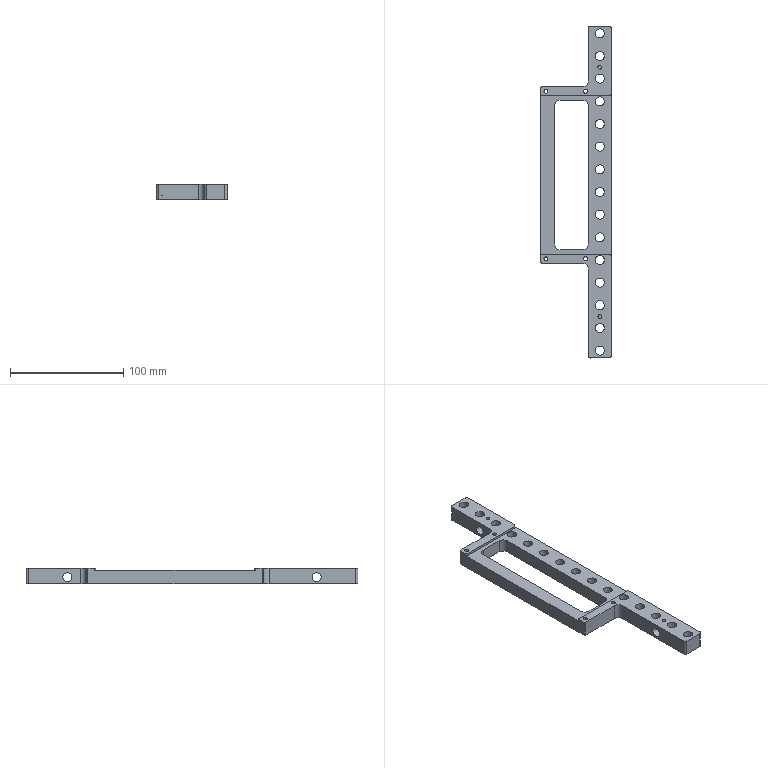Part | 1 solid | 80 faces | box 62 x 293 x 14 mm | volume 95449 mm3 | cylinder 58 | plane 22 | commonest cylinder face diameters 3.3 x17 8.1 x17 4 x6 10.2 x6 2 x4 3.5 x4